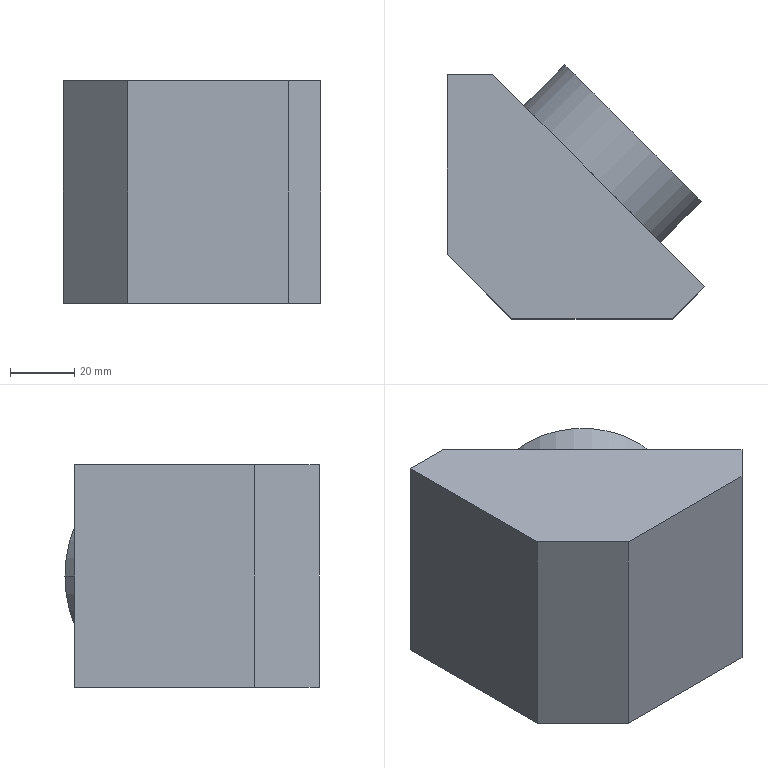Part | SolidWorks | features Chamfer 2, Extrusion 1, ICE 1 | 1 solid | 11 faces | box 80 x 78.941 x 69 mm | volume 302744 mm3 | plane 9 | cylinder 2 | commonest cylinder face diameters 60 x2
STEP:
#1=CARTESIAN_POINT('',(36.515,-11.059,34.5));
#2=VERTEX_POINT('',#1);
#3=CARTESIAN_POINT('',(78.941,-53.485,34.5));
#4=VERTEX_POINT('',#3);
#5=CARTESIAN_POINT('',(57.728,-32.272,34.5));
#6=DIRECTION('',(0.7071,0.7071,0.));
#7=DIRECTION('',(-0.7071,0.7071,0.));
#8=AXIS2_PLACEMENT_3D('',#5,#6,#7);
#9=CIRCLE('',#8,30.);
#10=EDGE_CURVE('',#2,#4,#9,.T.);
#11=ORIENTED_EDGE('',*,*,#10,.F.);
#12=CARTESIAN_POINT('',(23.787,-23.787,34.5));
#13=VERTEX_POINT('',#12);
#14=CARTESIAN_POINT('',(36.515,-11.059,34.5));
#15=DIRECTION('',(-0.7071,-0.7071,0.));
#16=VECTOR('',#15,1000.);
#17=LINE('',#14,#16);
#18=EDGE_CURVE('',#2,#13,#17,.T.);
#19=ORIENTED_EDGE('',*,*,#18,.T.);
#20=CARTESIAN_POINT('',(66.213,-66.213,34.5));
#21=VERTEX_POINT('',#20);
#22=CARTESIAN_POINT('',(45.,-45.,34.5));
#23=DIRECTION('',(0.7071,0.7071,0.));
#24=DIRECTION('',(-0.7071,0.7071,0.));
#25=AXIS2_PLACEMENT_3D('',#22,#23,#24);
#26=CIRCLE('',#25,30.);
#27=EDGE_CURVE('',#13,#21,#26,.T.);
#28=ORIENTED_EDGE('',*,*,#27,.T.);
#29=CARTESIAN_POINT('',(78.941,-53.485,34.5));
#30=DIRECTION('',(-0.7071,-0.7071,0.));
#31=VECTOR('',#30,1000.);
#32=LINE('',#29,#31);
#33=EDGE_CURVE('',#4,#21,#32,.T.);
#34=ORIENTED_EDGE('',*,*,#33,.F.);
#35=EDGE_LOOP('',(#11,#19,#28,#34));
#36=FACE_OUTER_BOUND('',#35,.T.);
#37=CARTESIAN_POINT('',(57.728,-32.272,34.5));
#38=DIRECTION('',(-0.7071,-0.7071,0.));
#39=DIRECTION('',(0.7071,-0.7071,0.));
#40=AXIS2_PLACEMENT_3D('',#37,#38,#39);
#41=CYLINDRICAL_SURFACE('',#40,30.);
#42=ADVANCED_FACE('',(#36),#41,.T.);
#43=CARTESIAN_POINT('',(45.,-45.,34.5));
#44=DIRECTION('',(0.7071,0.7071,0.));
#45=DIRECTION('',(-0.7071,0.7071,0.));
#46=AXIS2_PLACEMENT_3D('',#43,#44,#45);
#47=CIRCLE('',#46,30.);
#48=EDGE_CURVE('',#21,#13,#47,.T.);
#49=ORIENTED_EDGE('',*,*,#48,.F.);
#50=ORIENTED_EDGE('',*,*,#27,.F.);
#51=EDGE_LOOP('',(#49,#50));
#52=FACE_BOUND('',#51,.T.);
#53=CARTESIAN_POINT('',(80.,-80.,69.));
#54=VERTEX_POINT('',#53);
#55=CARTESIAN_POINT('',(14.142,-14.142,69.));
#56=VERTEX_POINT('',#55);
#57=CARTESIAN_POINT('',(90.,-90.,69.));
#58=DIRECTION('',(-0.7071,0.7071,0.));
#59=VECTOR('',#58,1000.);
#60=LINE('',#57,#59);
#61=EDGE_CURVE('',#54,#56,#60,.T.);
#62=ORIENTED_EDGE('',*,*,#61,.F.);
#63=CARTESIAN_POINT('',(80.,-80.,0.));
#64=VERTEX_POINT('',#63);
#65=CARTESIAN_POINT('',(80.,-80.,69.));
#66=DIRECTION('',(0.,0.,-1.));
#67=VECTOR('',#66,1000.);
#68=LINE('',#65,#67);
#69=EDGE_CURVE('',#54,#64,#68,.T.);
#70=ORIENTED_EDGE('',*,*,#69,.T.);
#71=CARTESIAN_POINT('',(14.142,-14.142,0.));
#72=VERTEX_POINT('',#71);
#73=CARTESIAN_POINT('',(90.,-90.,0.));
#74=DIRECTION('',(-0.7071,0.7071,0.));
#75=VECTOR('',#74,1000.);
#76=LINE('',#73,#75);
#77=EDGE_CURVE('',#64,#72,#76,.T.);
#78=ORIENTED_EDGE('',*,*,#77,.T.);
#79=CARTESIAN_POINT('',(14.142,-14.142,69.));
#80=DIRECTION('',(0.,0.,1.));
#81=VECTOR('',#80,1000.);
#82=LINE('',#79,#81);
#83=EDGE_CURVE('',#72,#56,#82,.T.);
#84=ORIENTED_EDGE('',*,*,#83,.T.);
#85=EDGE_LOOP('',(#62,#70,#78,#84));
#86=FACE_OUTER_BOUND('',#85,.T.);
#87=CARTESIAN_POINT('',(90.,-90.,69.));
#88=DIRECTION('',(-0.7071,-0.7071,0.));
#89=DIRECTION('',(0.7071,-0.7071,0.));
#90=AXIS2_PLACEMENT_3D('',#87,#88,#89);
#91=PLANE('',#90);
#92=ADVANCED_FACE('',(#52,#86),#91,.F.);
#93=CARTESIAN_POINT('',(0.,-14.142,69.));
#94=VERTEX_POINT('',#93);
#95=CARTESIAN_POINT('',(0.,-70.,69.));
#96=VERTEX_POINT('',#95);
#97=CARTESIAN_POINT('',(0.,0.,69.));
#98=DIRECTION('',(0.,-1.,0.));
#99=VECTOR('',#98,1000.);
#100=LINE('',#97,#99);
#101=EDGE_CURVE('',#94,#96,#100,.T.);
#102=ORIENTED_EDGE('',*,*,#101,.F.);
#103=CARTESIAN_POINT('',(0.,-14.142,0.));
#104=VERTEX_POINT('',#103);
#105=CARTESIAN_POINT('',(0.,-14.142,69.));
#106=DIRECTION('',(0.,0.,-1.));
#107=VECTOR('',#106,1000.);
#108=LINE('',#105,#107);
#109=EDGE_CURVE('',#94,#104,#108,.T.);
#110=ORIENTED_EDGE('',*,*,#109,.T.);
#111=CARTESIAN_POINT('',(0.,-70.,0.));
#112=VERTEX_POINT('',#111);
#113=CARTESIAN_POINT('',(0.,0.,0.));
#114=DIRECTION('',(0.,-1.,0.));
#115=VECTOR('',#114,1000.);
#116=LINE('',#113,#115);
#117=EDGE_CURVE('',#104,#112,#116,.T.);
#118=ORIENTED_EDGE('',*,*,#117,.T.);
#119=CARTESIAN_POINT('',(0.,-70.,69.));
#120=DIRECTION('',(0.,0.,1.));
#121=VECTOR('',#120,1000.);
#122=LINE('',#119,#121);
#123=EDGE_CURVE('',#112,#96,#122,.T.);
#124=ORIENTED_EDGE('',*,*,#123,.T.);
#125=EDGE_LOOP('',(#102,#110,#118,#124));
#126=FACE_OUTER_BOUND('',#125,.T.);
#127=CARTESIAN_POINT('',(0.,0.,69.));
#128=DIRECTION('',(1.,0.,0.));
#129=DIRECTION('',(0.,1.,0.));
#130=AXIS2_PLACEMENT_3D('',#127,#128,#129);
#131=PLANE('',#130);
#132=ADVANCED_FACE('',(#126),#131,.F.);
#133=CARTESIAN_POINT('',(20.,-90.,0.));
#134=VERTEX_POINT('',#133);
#135=CARTESIAN_POINT('',(70.,-90.,0.));
#136=VERTEX_POINT('',#135);
#137=CARTESIAN_POINT('',(0.,-90.,0.));
#138=DIRECTION('',(1.,0.,0.));
#139=VECTOR('',#138,1000.);
#140=LINE('',#137,#139);
#141=EDGE_CURVE('',#134,#136,#140,.T.);
#142=ORIENTED_EDGE('',*,*,#141,.T.);
#143=CARTESIAN_POINT('',(70.,-90.,69.));
#144=VERTEX_POINT('',#143);
#145=CARTESIAN_POINT('',(70.,-90.,69.));
#146=DIRECTION('',(0.,0.,1.));
#147=VECTOR('',#146,1000.);
#148=LINE('',#145,#147);
#149=EDGE_CURVE('',#136,#144,#148,.T.);
#150=ORIENTED_EDGE('',*,*,#149,.T.);
#151=CARTESIAN_POINT('',(20.,-90.,69.));
#152=VERTEX_POINT('',#151);
#153=CARTESIAN_POINT('',(0.,-90.,69.));
#154=DIRECTION('',(1.,0.,0.));
#155=VECTOR('',#154,1000.);
#156=LINE('',#153,#155);
#157=EDGE_CURVE('',#152,#144,#156,.T.);
#158=ORIENTED_EDGE('',*,*,#157,.F.);
#159=CARTESIAN_POINT('',(20.,-90.,69.));
#160=DIRECTION('',(0.,0.,-1.));
#161=VECTOR('',#160,1000.);
#162=LINE('',#159,#161);
#163=EDGE_CURVE('',#152,#134,#162,.T.);
#164=ORIENTED_EDGE('',*,*,#163,.T.);
#165=EDGE_LOOP('',(#142,#150,#158,#164));
#166=FACE_OUTER_BOUND('',#165,.T.);
#167=CARTESIAN_POINT('',(0.,-90.,69.));
#168=DIRECTION('',(0.,1.,0.));
#169=DIRECTION('',(0.,0.,1.));
#170=AXIS2_PLACEMENT_3D('',#167,#168,#169);
#171=PLANE('',#170);
#172=ADVANCED_FACE('',(#166),#171,.F.);
#173=ORIENTED_EDGE('',*,*,#157,.T.);
#174=CARTESIAN_POINT('',(80.,-80.,69.));
#175=DIRECTION('',(0.7071,0.7071,0.));
#176=VECTOR('',#175,1000.);
#177=LINE('',#174,#176);
#178=EDGE_CURVE('',#144,#54,#177,.T.);
#179=ORIENTED_EDGE('',*,*,#178,.T.);
#180=ORIENTED_EDGE('',*,*,#61,.T.);
#181=CARTESIAN_POINT('',(0.,-14.142,69.));
#182=DIRECTION('',(-1.,0.,0.));
#183=VECTOR('',#182,1000.);
#184=LINE('',#181,#183);
#185=EDGE_CURVE('',#56,#94,#184,.T.);
#186=ORIENTED_EDGE('',*,*,#185,.T.);
#187=ORIENTED_EDGE('',*,*,#101,.T.);
#188=CARTESIAN_POINT('',(-35.,-35.,69.));
#189=DIRECTION('',(0.7071,-0.7071,0.));
#190=VECTOR('',#189,1000.);
#191=LINE('',#188,#190);
#192=EDGE_CURVE('',#96,#152,#191,.T.);
#193=ORIENTED_EDGE('',*,*,#192,.T.);
#194=EDGE_LOOP('',(#173,#179,#180,#186,#187,#193));
#195=FACE_OUTER_BOUND('',#194,.T.);
#196=CARTESIAN_POINT('',(0.,0.,69.));
#197=DIRECTION('',(0.,0.,1.));
#198=DIRECTION('',(1.,0.,0.));
#199=AXIS2_PLACEMENT_3D('',#196,#197,#198);
#200=PLANE('',#199);
#201=ADVANCED_FACE('',(#195),#200,.T.);
#202=ORIENTED_EDGE('',*,*,#77,.F.);
#203=CARTESIAN_POINT('',(80.,-80.,0.));
#204=DIRECTION('',(-0.7071,-0.7071,0.));
#205=VECTOR('',#204,1000.);
#206=LINE('',#203,#205);
#207=EDGE_CURVE('',#64,#136,#206,.T.);
#208=ORIENTED_EDGE('',*,*,#207,.T.);
#209=ORIENTED_EDGE('',*,*,#141,.F.);
#210=CARTESIAN_POINT('',(20.,-90.,0.));
#211=DIRECTION('',(-0.7071,0.7071,0.));
#212=VECTOR('',#211,1000.);
#213=LINE('',#210,#212);
#214=EDGE_CURVE('',#134,#112,#213,.T.);
#215=ORIENTED_EDGE('',*,*,#214,.T.);
#216=ORIENTED_EDGE('',*,*,#117,.F.);
#217=CARTESIAN_POINT('',(0.,-14.142,0.));
#218=DIRECTION('',(1.,0.,0.));
#219=VECTOR('',#218,1000.);
#220=LINE('',#217,#219);
#221=EDGE_CURVE('',#104,#72,#220,.T.);
#222=ORIENTED_EDGE('',*,*,#221,.T.);
#223=EDGE_LOOP('',(#202,#208,#209,#215,#216,#222));
#224=FACE_OUTER_BOUND('',#223,.T.);
#225=CARTESIAN_POINT('',(0.,0.,0.));
#226=DIRECTION('',(0.,0.,1.));
#227=DIRECTION('',(1.,0.,0.));
#228=AXIS2_PLACEMENT_3D('',#225,#226,#227);
#229=PLANE('',#228);
#230=ADVANCED_FACE('',(#224),#229,.F.);
#231=ORIENTED_EDGE('',*,*,#192,.F.);
#232=ORIENTED_EDGE('',*,*,#123,.F.);
#233=ORIENTED_EDGE('',*,*,#214,.F.);
#234=ORIENTED_EDGE('',*,*,#163,.F.);
#235=EDGE_LOOP('',(#231,#232,#233,#234));
#236=FACE_OUTER_BOUND('',#235,.T.);
#237=CARTESIAN_POINT('',(20.,-90.,69.));
#238=DIRECTION('',(0.7071,0.7071,0.));
#239=DIRECTION('',(0.,0.,-1.));
#240=AXIS2_PLACEMENT_3D('',#237,#238,#239);
#241=PLANE('',#240);
#242=ADVANCED_FACE('',(#236),#241,.F.);
#243=ORIENTED_EDGE('',*,*,#18,.F.);
#244=CARTESIAN_POINT('',(57.728,-32.272,34.5));
#245=DIRECTION('',(0.7071,0.7071,0.));
#246=DIRECTION('',(-0.7071,0.7071,0.));
#247=AXIS2_PLACEMENT_3D('',#244,#245,#246);
#248=CIRCLE('',#247,30.);
#249=EDGE_CURVE('',#4,#2,#248,.T.);
#250=ORIENTED_EDGE('',*,*,#249,.F.);
#251=ORIENTED_EDGE('',*,*,#33,.T.);
#252=ORIENTED_EDGE('',*,*,#48,.T.);
#253=EDGE_LOOP('',(#243,#250,#251,#252));
#254=FACE_OUTER_BOUND('',#253,.T.);
#255=CARTESIAN_POINT('',(57.728,-32.272,34.5));
#256=DIRECTION('',(-0.7071,-0.7071,0.));
#257=DIRECTION('',(0.7071,-0.7071,0.));
#258=AXIS2_PLACEMENT_3D('',#255,#256,#257);
#259=CYLINDRICAL_SURFACE('',#258,30.);
#260=ADVANCED_FACE('',(#254),#259,.T.);
#261=ORIENTED_EDGE('',*,*,#249,.T.);
#262=ORIENTED_EDGE('',*,*,#10,.T.);
#263=EDGE_LOOP('',(#261,#262));
#264=FACE_OUTER_BOUND('',#263,.T.);
#265=CARTESIAN_POINT('',(57.728,-32.272,34.5));
#266=DIRECTION('',(0.7071,0.7071,0.));
#267=DIRECTION('',(-0.7071,0.7071,0.));
#268=AXIS2_PLACEMENT_3D('',#265,#266,#267);
#269=PLANE('',#268);
#270=ADVANCED_FACE('',(#264),#269,.T.);
#271=ORIENTED_EDGE('',*,*,#178,.F.);
#272=ORIENTED_EDGE('',*,*,#149,.F.);
#273=ORIENTED_EDGE('',*,*,#207,.F.);
#274=ORIENTED_EDGE('',*,*,#69,.F.);
#275=EDGE_LOOP('',(#271,#272,#273,#274));
#276=FACE_OUTER_BOUND('',#275,.T.);
#277=CARTESIAN_POINT('',(80.,-80.,69.));
#278=DIRECTION('',(-0.7071,0.7071,0.));
#279=DIRECTION('',(0.,0.,-1.));
#280=AXIS2_PLACEMENT_3D('',#277,#278,#279);
#281=PLANE('',#280);
#282=ADVANCED_FACE('',(#276),#281,.F.);
#283=ORIENTED_EDGE('',*,*,#185,.F.);
#284=ORIENTED_EDGE('',*,*,#83,.F.);
#285=ORIENTED_EDGE('',*,*,#221,.F.);
#286=ORIENTED_EDGE('',*,*,#109,.F.);
#287=EDGE_LOOP('',(#283,#284,#285,#286));
#288=FACE_OUTER_BOUND('',#287,.T.);
#289=CARTESIAN_POINT('',(0.,-14.142,69.));
#290=DIRECTION('',(0.,-1.,0.));
#291=DIRECTION('',(0.,0.,-1.));
#292=AXIS2_PLACEMENT_3D('',#289,#290,#291);
#293=PLANE('',#292);
#294=ADVANCED_FACE('',(#288),#293,.F.);
#295=CLOSED_SHELL('',(#42,#92,#132,#172,#201,#230,#242,#260,#270,#282,#294));
#296=MANIFOLD_SOLID_BREP('',#295);
#297=CARTESIAN_POINT('',(0.,0.,0.));
#298=DIRECTION('',(0.,0.,1.));
#299=DIRECTION('',(1.,0.,0.));
#300=AXIS2_PLACEMENT_3D('',#297,#298,#299);
#301=(LENGTH_UNIT()NAMED_UNIT(*)SI_UNIT(.MILLI.,.METRE.));
#302=UNCERTAINTY_MEASURE_WITH_UNIT(LENGTH_MEASURE(0.00001),#301,'','');
#303=(NAMED_UNIT(*)PLANE_ANGLE_UNIT()SI_UNIT($,.RADIAN.));
#304=(NAMED_UNIT(*)SI_UNIT($,.STERADIAN.)SOLID_ANGLE_UNIT());
#305=(GEOMETRIC_REPRESENTATION_CONTEXT(3)GLOBAL_UNCERTAINTY_ASSIGNED_CONTEXT((#302))GLOBAL_UNIT_ASSIGNED_CONTEXT((#301,#303,#304))REPRESENTATION_CONTEXT('',''));
#306=ADVANCED_BREP_SHAPE_REPRESENTATION('',(#296,#300),#305);